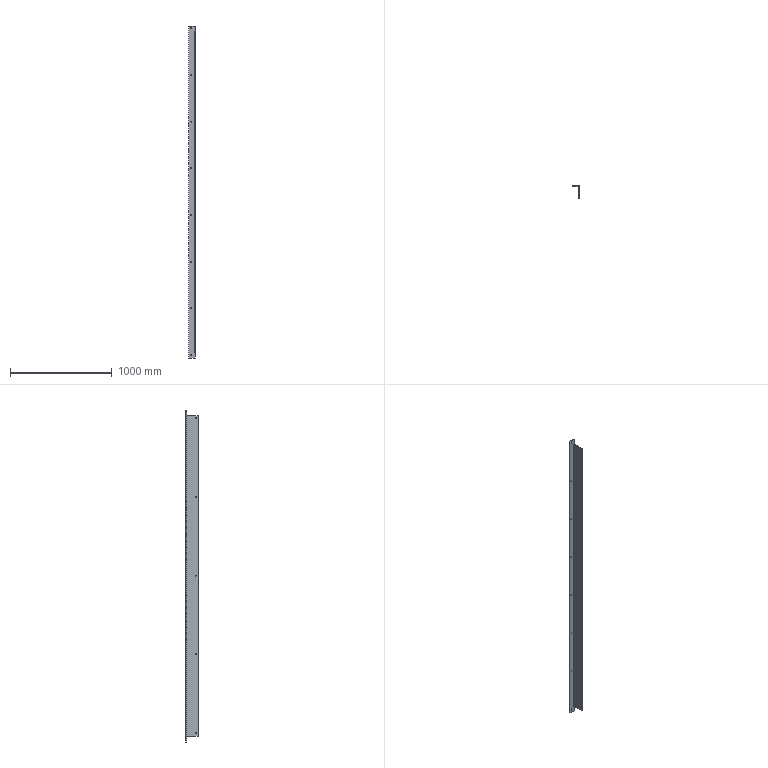Part | SolidWorks | features BaseBody 1 | 1 solid | 60 faces | box 60 x 120 x 3271 mm | volume 3298320 mm3 | cylinder 28 | cone 16 | plane 16 | commonest cylinder face diameters 9 x26 1.473 x1 13.473 x1